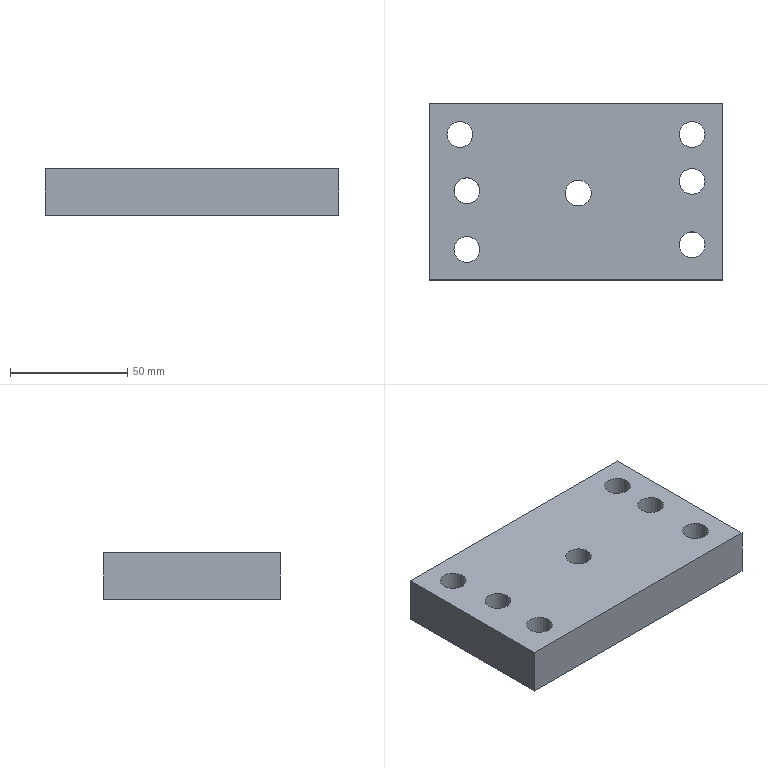Part | STEP file | 113_id2782_x_t | 1 solid | 13 faces | box 125 x 75 x 20 mm | volume 174195 mm3 | cylinder 7 | plane 6 | commonest cylinder face diameters 11 x7
STEP:
#1=CARTESIAN_POINT('',(0.,0.,0.));
#2=DIRECTION('',(0.,0.,1.));
#3=DIRECTION('',(1.,0.,0.));
#4=AXIS2_PLACEMENT_3D('',#1,#2,#3);
#5=CARTESIAN_POINT('',(1103.,139.,85.));
#6=VERTEX_POINT('',#5);
#7=CARTESIAN_POINT('',(1114.,139.,85.));
#8=VERTEX_POINT('',#7);
#9=CARTESIAN_POINT('',(1108.5,139.,85.));
#10=DIRECTION('',(0.,0.,1.));
#11=DIRECTION('',(-1.,0.,0.));
#12=AXIS2_PLACEMENT_3D('',#9,#10,#11);
#13=CIRCLE('',#12,5.5);
#14=CARTESIAN_POINT('',(1128.,155.,85.));
#15=DIRECTION('',(0.,0.,-1.));
#16=DIRECTION('',(1.,0.,0.));
#17=AXIS2_PLACEMENT_3D('',#14,#15,#16);
#18=PLANE('',#17);
#19=CARTESIAN_POINT('',(-25.,16.));
#20=CARTESIAN_POINT('',(-25.,25.526));
#21=CARTESIAN_POINT('',(-16.75,20.763));
#22=CARTESIAN_POINT('',(-8.5,16.));
#23=CARTESIAN_POINT('',(-16.75,11.237));
#24=CARTESIAN_POINT('',(-25.,6.474));
#25=CARTESIAN_POINT('',(-25.,16.));
#26=(BOUNDED_CURVE()B_SPLINE_CURVE(2,(#19,#20,#21,#22,#23,#24,#25),.UNSPECIFIED.,.T.,.F.)B_SPLINE_CURVE_WITH_KNOTS((1,2,2,2,2,1),(-2.094,0.,2.094,4.189,6.283,8.378),.UNSPECIFIED.)CURVE()GEOMETRIC_REPRESENTATION_ITEM()RATIONAL_B_SPLINE_CURVE((1.,0.5,1.,0.5,1.,0.5,1.))REPRESENTATION_ITEM(''));
#27=(GEOMETRIC_REPRESENTATION_CONTEXT(2)PARAMETRIC_REPRESENTATION_CONTEXT()REPRESENTATION_CONTEXT('',''));
#28=DEFINITIONAL_REPRESENTATION('',(#26),#27);
#29=PCURVE('',#18,#28);
#30=CARTESIAN_POINT('',(1108.5,139.,215.));
#31=DIRECTION('',(0.,0.,-1.));
#32=DIRECTION('',(1.,0.,0.));
#33=AXIS2_PLACEMENT_3D('',#30,#31,#32);
#34=CYLINDRICAL_SURFACE('',#33,5.5);
#35=CARTESIAN_POINT('',(3.142,130.));
#36=DIRECTION('',(-1.,0.));
#37=VECTOR('',#36,1.);
#38=LINE('',#35,#37);
#39=(GEOMETRIC_REPRESENTATION_CONTEXT(2)PARAMETRIC_REPRESENTATION_CONTEXT()REPRESENTATION_CONTEXT('',''));
#40=DEFINITIONAL_REPRESENTATION('',(#38),#39);
#41=PCURVE('',#34,#40);
#42=SURFACE_CURVE('',#13,(#29,#41),.PCURVE_S1.);
#43=EDGE_CURVE('',#6,#8,#42,.T.);
#44=ORIENTED_EDGE('',*,*,#43,.T.);
#45=CARTESIAN_POINT('',(1108.5,139.,85.));
#46=DIRECTION('',(0.,0.,1.));
#47=DIRECTION('',(-1.,0.,0.));
#48=AXIS2_PLACEMENT_3D('',#45,#46,#47);
#49=CIRCLE('',#48,5.5);
#50=CARTESIAN_POINT('',(-25.,16.));
#51=CARTESIAN_POINT('',(-25.,25.526));
#52=CARTESIAN_POINT('',(-16.75,20.763));
#53=CARTESIAN_POINT('',(-8.5,16.));
#54=CARTESIAN_POINT('',(-16.75,11.237));
#55=CARTESIAN_POINT('',(-25.,6.474));
#56=CARTESIAN_POINT('',(-25.,16.));
#57=(BOUNDED_CURVE()B_SPLINE_CURVE(2,(#50,#51,#52,#53,#54,#55,#56),.UNSPECIFIED.,.T.,.F.)B_SPLINE_CURVE_WITH_KNOTS((1,2,2,2,2,1),(-2.094,0.,2.094,4.189,6.283,8.378),.UNSPECIFIED.)CURVE()GEOMETRIC_REPRESENTATION_ITEM()RATIONAL_B_SPLINE_CURVE((1.,0.5,1.,0.5,1.,0.5,1.))REPRESENTATION_ITEM(''));
#58=(GEOMETRIC_REPRESENTATION_CONTEXT(2)PARAMETRIC_REPRESENTATION_CONTEXT()REPRESENTATION_CONTEXT('',''));
#59=DEFINITIONAL_REPRESENTATION('',(#57),#58);
#60=PCURVE('',#18,#59);
#61=CARTESIAN_POINT('',(9.425,130.));
#62=DIRECTION('',(-1.,0.));
#63=VECTOR('',#62,1.);
#64=LINE('',#61,#63);
#65=(GEOMETRIC_REPRESENTATION_CONTEXT(2)PARAMETRIC_REPRESENTATION_CONTEXT()REPRESENTATION_CONTEXT('',''));
#66=DEFINITIONAL_REPRESENTATION('',(#64),#65);
#67=PCURVE('',#34,#66);
#68=SURFACE_CURVE('',#49,(#60,#67),.PCURVE_S1.);
#69=EDGE_CURVE('',#8,#6,#68,.T.);
#70=ORIENTED_EDGE('',*,*,#69,.T.);
#71=EDGE_LOOP('',(#44,#70));
#72=FACE_BOUND('',#71,.T.);
#73=CARTESIAN_POINT('',(1054.5,161.,85.));
#74=VERTEX_POINT('',#73);
#75=CARTESIAN_POINT('',(1065.5,161.,85.));
#76=VERTEX_POINT('',#75);
#77=CARTESIAN_POINT('',(1060.,161.,85.));
#78=DIRECTION('',(0.,0.,1.));
#79=DIRECTION('',(-1.,0.,0.));
#80=AXIS2_PLACEMENT_3D('',#77,#78,#79);
#81=CIRCLE('',#80,5.5);
#82=CARTESIAN_POINT('',(-73.5,-6.));
#83=CARTESIAN_POINT('',(-73.5,3.526));
#84=CARTESIAN_POINT('',(-65.25,-1.237));
#85=CARTESIAN_POINT('',(-57.,-6.));
#86=CARTESIAN_POINT('',(-65.25,-10.763));
#87=CARTESIAN_POINT('',(-73.5,-15.526));
#88=CARTESIAN_POINT('',(-73.5,-6.));
#89=(BOUNDED_CURVE()B_SPLINE_CURVE(2,(#82,#83,#84,#85,#86,#87,#88),.UNSPECIFIED.,.T.,.F.)B_SPLINE_CURVE_WITH_KNOTS((1,2,2,2,2,1),(-2.094,0.,2.094,4.189,6.283,8.378),.UNSPECIFIED.)CURVE()GEOMETRIC_REPRESENTATION_ITEM()RATIONAL_B_SPLINE_CURVE((1.,0.5,1.,0.5,1.,0.5,1.))REPRESENTATION_ITEM(''));
#90=(GEOMETRIC_REPRESENTATION_CONTEXT(2)PARAMETRIC_REPRESENTATION_CONTEXT()REPRESENTATION_CONTEXT('',''));
#91=DEFINITIONAL_REPRESENTATION('',(#89),#90);
#92=PCURVE('',#18,#91);
#93=CARTESIAN_POINT('',(1060.,161.,190.));
#94=DIRECTION('',(0.,0.,-1.));
#95=DIRECTION('',(1.,0.,0.));
#96=AXIS2_PLACEMENT_3D('',#93,#94,#95);
#97=CYLINDRICAL_SURFACE('',#96,5.5);
#98=CARTESIAN_POINT('',(3.142,105.));
#99=DIRECTION('',(-1.,0.));
#100=VECTOR('',#99,1.);
#101=LINE('',#98,#100);
#102=(GEOMETRIC_REPRESENTATION_CONTEXT(2)PARAMETRIC_REPRESENTATION_CONTEXT()REPRESENTATION_CONTEXT('',''));
#103=DEFINITIONAL_REPRESENTATION('',(#101),#102);
#104=PCURVE('',#97,#103);
#105=SURFACE_CURVE('',#81,(#92,#104),.PCURVE_S1.);
#106=EDGE_CURVE('',#74,#76,#105,.T.);
#107=ORIENTED_EDGE('',*,*,#106,.T.);
#108=CARTESIAN_POINT('',(1060.,161.,85.));
#109=DIRECTION('',(0.,0.,1.));
#110=DIRECTION('',(-1.,0.,0.));
#111=AXIS2_PLACEMENT_3D('',#108,#109,#110);
#112=CIRCLE('',#111,5.5);
#113=CARTESIAN_POINT('',(-73.5,-6.));
#114=CARTESIAN_POINT('',(-73.5,3.526));
#115=CARTESIAN_POINT('',(-65.25,-1.237));
#116=CARTESIAN_POINT('',(-57.,-6.));
#117=CARTESIAN_POINT('',(-65.25,-10.763));
#118=CARTESIAN_POINT('',(-73.5,-15.526));
#119=CARTESIAN_POINT('',(-73.5,-6.));
#120=(BOUNDED_CURVE()B_SPLINE_CURVE(2,(#113,#114,#115,#116,#117,#118,#119),.UNSPECIFIED.,.T.,.F.)B_SPLINE_CURVE_WITH_KNOTS((1,2,2,2,2,1),(-2.094,0.,2.094,4.189,6.283,8.378),.UNSPECIFIED.)CURVE()GEOMETRIC_REPRESENTATION_ITEM()RATIONAL_B_SPLINE_CURVE((1.,0.5,1.,0.5,1.,0.5,1.))REPRESENTATION_ITEM(''));
#121=(GEOMETRIC_REPRESENTATION_CONTEXT(2)PARAMETRIC_REPRESENTATION_CONTEXT()REPRESENTATION_CONTEXT('',''));
#122=DEFINITIONAL_REPRESENTATION('',(#120),#121);
#123=PCURVE('',#18,#122);
#124=CARTESIAN_POINT('',(9.425,105.));
#125=DIRECTION('',(-1.,0.));
#126=VECTOR('',#125,1.);
#127=LINE('',#124,#126);
#128=(GEOMETRIC_REPRESENTATION_CONTEXT(2)PARAMETRIC_REPRESENTATION_CONTEXT()REPRESENTATION_CONTEXT('',''));
#129=DEFINITIONAL_REPRESENTATION('',(#127),#128);
#130=PCURVE('',#97,#129);
#131=SURFACE_CURVE('',#112,(#123,#130),.PCURVE_S1.);
#132=EDGE_CURVE('',#76,#74,#131,.T.);
#133=ORIENTED_EDGE('',*,*,#132,.T.);
#134=EDGE_LOOP('',(#107,#133));
#135=FACE_BOUND('',#134,.T.);
#136=CARTESIAN_POINT('',(1018.,137.,85.));
#137=VERTEX_POINT('',#136);
#138=CARTESIAN_POINT('',(1012.5,137.,85.));
#139=DIRECTION('',(0.,0.,1.));
#140=DIRECTION('',(-1.,0.,0.));
#141=AXIS2_PLACEMENT_3D('',#138,#139,#140);
#142=CIRCLE('',#141,5.5);
#143=CARTESIAN_POINT('',(-121.,18.));
#144=CARTESIAN_POINT('',(-121.,27.526));
#145=CARTESIAN_POINT('',(-112.75,22.763));
#146=CARTESIAN_POINT('',(-104.5,18.));
#147=CARTESIAN_POINT('',(-112.75,13.237));
#148=CARTESIAN_POINT('',(-121.,8.474));
#149=CARTESIAN_POINT('',(-121.,18.));
#150=(BOUNDED_CURVE()B_SPLINE_CURVE(2,(#143,#144,#145,#146,#147,#148,#149),.UNSPECIFIED.,.T.,.F.)B_SPLINE_CURVE_WITH_KNOTS((1,2,2,2,2,1),(-2.094,0.,2.094,4.189,6.283,8.378),.UNSPECIFIED.)CURVE()GEOMETRIC_REPRESENTATION_ITEM()RATIONAL_B_SPLINE_CURVE((1.,0.5,1.,0.5,1.,0.5,1.))REPRESENTATION_ITEM(''));
#151=(GEOMETRIC_REPRESENTATION_CONTEXT(2)PARAMETRIC_REPRESENTATION_CONTEXT()REPRESENTATION_CONTEXT('',''));
#152=DEFINITIONAL_REPRESENTATION('',(#150),#151);
#153=PCURVE('',#18,#152);
#154=CARTESIAN_POINT('',(1012.5,137.,90.));
#155=DIRECTION('',(0.,0.,1.));
#156=DIRECTION('',(-1.,0.,0.));
#157=AXIS2_PLACEMENT_3D('',#154,#155,#156);
#158=CYLINDRICAL_SURFACE('',#157,5.5);
#159=CARTESIAN_POINT('',(0.,-5.));
#160=DIRECTION('',(1.,0.));
#161=VECTOR('',#160,1.);
#162=LINE('',#159,#161);
#163=(GEOMETRIC_REPRESENTATION_CONTEXT(2)PARAMETRIC_REPRESENTATION_CONTEXT()REPRESENTATION_CONTEXT('',''));
#164=DEFINITIONAL_REPRESENTATION('',(#162),#163);
#165=PCURVE('',#158,#164);
#166=SURFACE_CURVE('',#142,(#153,#165),.PCURVE_S1.);
#167=EDGE_CURVE('',#137,#137,#166,.T.);
#168=ORIENTED_EDGE('',*,*,#167,.T.);
#169=EDGE_LOOP('',(#168));
#170=FACE_BOUND('',#169,.T.);
#171=CARTESIAN_POINT('',(1012.5,167.5,85.));
#172=VERTEX_POINT('',#171);
#173=CARTESIAN_POINT('',(1018.,162.,85.));
#174=VERTEX_POINT('',#173);
#175=CARTESIAN_POINT('',(1012.5,162.,85.));
#176=DIRECTION('',(0.,0.,1.));
#177=DIRECTION('',(-1.,0.,0.));
#178=AXIS2_PLACEMENT_3D('',#175,#176,#177);
#179=CIRCLE('',#178,5.5);
#180=CARTESIAN_POINT('',(-121.,-7.));
#181=CARTESIAN_POINT('',(-121.,2.526));
#182=CARTESIAN_POINT('',(-112.75,-2.237));
#183=CARTESIAN_POINT('',(-104.5,-7.));
#184=CARTESIAN_POINT('',(-112.75,-11.763));
#185=CARTESIAN_POINT('',(-121.,-16.526));
#186=CARTESIAN_POINT('',(-121.,-7.));
#187=(BOUNDED_CURVE()B_SPLINE_CURVE(2,(#180,#181,#182,#183,#184,#185,#186),.UNSPECIFIED.,.T.,.F.)B_SPLINE_CURVE_WITH_KNOTS((1,2,2,2,2,1),(-2.094,0.,2.094,4.189,6.283,8.378),.UNSPECIFIED.)CURVE()GEOMETRIC_REPRESENTATION_ITEM()RATIONAL_B_SPLINE_CURVE((1.,0.5,1.,0.5,1.,0.5,1.))REPRESENTATION_ITEM(''));
#188=(GEOMETRIC_REPRESENTATION_CONTEXT(2)PARAMETRIC_REPRESENTATION_CONTEXT()REPRESENTATION_CONTEXT('',''));
#189=DEFINITIONAL_REPRESENTATION('',(#187),#188);
#190=PCURVE('',#18,#189);
#191=CARTESIAN_POINT('',(1012.5,162.,90.));
#192=DIRECTION('',(0.,0.,1.));
#193=DIRECTION('',(0.,-1.,0.));
#194=AXIS2_PLACEMENT_3D('',#191,#192,#193);
#195=CYLINDRICAL_SURFACE('',#194,5.5);
#196=CARTESIAN_POINT('',(-1.571,-5.));
#197=DIRECTION('',(1.,0.));
#198=VECTOR('',#197,1.);
#199=LINE('',#196,#198);
#200=(GEOMETRIC_REPRESENTATION_CONTEXT(2)PARAMETRIC_REPRESENTATION_CONTEXT()REPRESENTATION_CONTEXT('',''));
#201=DEFINITIONAL_REPRESENTATION('',(#199),#200);
#202=PCURVE('',#195,#201);
#203=SURFACE_CURVE('',#179,(#190,#202),.PCURVE_S1.);
#204=EDGE_CURVE('',#172,#174,#203,.T.);
#205=ORIENTED_EDGE('',*,*,#204,.T.);
#206=CARTESIAN_POINT('',(1012.5,162.,85.));
#207=DIRECTION('',(0.,0.,1.));
#208=DIRECTION('',(-1.,0.,0.));
#209=AXIS2_PLACEMENT_3D('',#206,#207,#208);
#210=CIRCLE('',#209,5.5);
#211=CARTESIAN_POINT('',(-121.,-7.));
#212=CARTESIAN_POINT('',(-121.,2.526));
#213=CARTESIAN_POINT('',(-112.75,-2.237));
#214=CARTESIAN_POINT('',(-104.5,-7.));
#215=CARTESIAN_POINT('',(-112.75,-11.763));
#216=CARTESIAN_POINT('',(-121.,-16.526));
#217=CARTESIAN_POINT('',(-121.,-7.));
#218=(BOUNDED_CURVE()B_SPLINE_CURVE(2,(#211,#212,#213,#214,#215,#216,#217),.UNSPECIFIED.,.T.,.F.)B_SPLINE_CURVE_WITH_KNOTS((1,2,2,2,2,1),(-2.094,0.,2.094,4.189,6.283,8.378),.UNSPECIFIED.)CURVE()GEOMETRIC_REPRESENTATION_ITEM()RATIONAL_B_SPLINE_CURVE((1.,0.5,1.,0.5,1.,0.5,1.))REPRESENTATION_ITEM(''));
#219=(GEOMETRIC_REPRESENTATION_CONTEXT(2)PARAMETRIC_REPRESENTATION_CONTEXT()REPRESENTATION_CONTEXT('',''));
#220=DEFINITIONAL_REPRESENTATION('',(#218),#219);
#221=PCURVE('',#18,#220);
#222=CARTESIAN_POINT('',(-1.571,-5.));
#223=DIRECTION('',(1.,0.));
#224=VECTOR('',#223,1.);
#225=LINE('',#222,#224);
#226=(GEOMETRIC_REPRESENTATION_CONTEXT(2)PARAMETRIC_REPRESENTATION_CONTEXT()REPRESENTATION_CONTEXT('',''));
#227=DEFINITIONAL_REPRESENTATION('',(#225),#226);
#228=PCURVE('',#195,#227);
#229=SURFACE_CURVE('',#210,(#221,#228),.PCURVE_S1.);
#230=EDGE_CURVE('',#174,#172,#229,.T.);
#231=ORIENTED_EDGE('',*,*,#230,.T.);
#232=EDGE_LOOP('',(#205,#231));
#233=FACE_BOUND('',#232,.T.);
#234=CARTESIAN_POINT('',(1015.,186.,85.));
#235=VERTEX_POINT('',#234);
#236=CARTESIAN_POINT('',(1009.5,186.,85.));
#237=DIRECTION('',(0.,0.,1.));
#238=DIRECTION('',(-1.,0.,0.));
#239=AXIS2_PLACEMENT_3D('',#236,#237,#238);
#240=CIRCLE('',#239,5.5);
#241=CARTESIAN_POINT('',(-124.,-31.));
#242=CARTESIAN_POINT('',(-124.,-21.474));
#243=CARTESIAN_POINT('',(-115.75,-26.237));
#244=CARTESIAN_POINT('',(-107.5,-31.));
#245=CARTESIAN_POINT('',(-115.75,-35.763));
#246=CARTESIAN_POINT('',(-124.,-40.526));
#247=CARTESIAN_POINT('',(-124.,-31.));
#248=(BOUNDED_CURVE()B_SPLINE_CURVE(2,(#241,#242,#243,#244,#245,#246,#247),.UNSPECIFIED.,.T.,.F.)B_SPLINE_CURVE_WITH_KNOTS((1,2,2,2,2,1),(-2.094,0.,2.094,4.189,6.283,8.378),.UNSPECIFIED.)CURVE()GEOMETRIC_REPRESENTATION_ITEM()RATIONAL_B_SPLINE_CURVE((1.,0.5,1.,0.5,1.,0.5,1.))REPRESENTATION_ITEM(''));
#249=(GEOMETRIC_REPRESENTATION_CONTEXT(2)PARAMETRIC_REPRESENTATION_CONTEXT()REPRESENTATION_CONTEXT('',''));
#250=DEFINITIONAL_REPRESENTATION('',(#248),#249);
#251=PCURVE('',#18,#250);
#252=CARTESIAN_POINT('',(1009.5,186.,90.));
#253=DIRECTION('',(0.,0.,1.));
#254=DIRECTION('',(-1.,0.,0.));
#255=AXIS2_PLACEMENT_3D('',#252,#253,#254);
#256=CYLINDRICAL_SURFACE('',#255,5.5);
#257=CARTESIAN_POINT('',(0.,-5.));
#258=DIRECTION('',(1.,0.));
#259=VECTOR('',#258,1.);
#260=LINE('',#257,#259);
#261=(GEOMETRIC_REPRESENTATION_CONTEXT(2)PARAMETRIC_REPRESENTATION_CONTEXT()REPRESENTATION_CONTEXT('',''));
#262=DEFINITIONAL_REPRESENTATION('',(#260),#261);
#263=PCURVE('',#256,#262);
#264=SURFACE_CURVE('',#240,(#251,#263),.PCURVE_S1.);
#265=EDGE_CURVE('',#235,#235,#264,.T.);
#266=ORIENTED_EDGE('',*,*,#265,.T.);
#267=EDGE_LOOP('',(#266));
#268=FACE_BOUND('',#267,.T.);
#269=CARTESIAN_POINT('',(1121.5,199.,85.));
#270=VERTEX_POINT('',#269);
#271=CARTESIAN_POINT('',(1121.5,124.,85.));
#272=VERTEX_POINT('',#271);
#273=CARTESIAN_POINT('',(1121.5,155.,85.));
#274=DIRECTION('',(0.,-1.,0.));
#275=VECTOR('',#274,1.);
#276=LINE('',#273,#275);
#277=CARTESIAN_POINT('',(-6.5,0.));
#278=DIRECTION('',(0.,1.));
#279=VECTOR('',#278,1.);
#280=LINE('',#277,#279);
#281=(GEOMETRIC_REPRESENTATION_CONTEXT(2)PARAMETRIC_REPRESENTATION_CONTEXT()REPRESENTATION_CONTEXT('',''));
#282=DEFINITIONAL_REPRESENTATION('',(#280),#281);
#283=PCURVE('',#18,#282);
#284=CARTESIAN_POINT('',(1121.5,161.,38.5));
#285=DIRECTION('',(1.,0.,0.));
#286=DIRECTION('',(0.,0.,1.));
#287=AXIS2_PLACEMENT_3D('',#284,#285,#286);
#288=PLANE('',#287);
#289=CARTESIAN_POINT('',(46.5,6.));
#290=DIRECTION('',(0.,1.));
#291=VECTOR('',#290,1.);
#292=LINE('',#289,#291);
#293=(GEOMETRIC_REPRESENTATION_CONTEXT(2)PARAMETRIC_REPRESENTATION_CONTEXT()REPRESENTATION_CONTEXT('',''));
#294=DEFINITIONAL_REPRESENTATION('',(#292),#293);
#295=PCURVE('',#288,#294);
#296=SURFACE_CURVE('',#276,(#283,#295),.PCURVE_S1.);
#297=EDGE_CURVE('',#270,#272,#296,.T.);
#298=ORIENTED_EDGE('',*,*,#297,.T.);
#299=CARTESIAN_POINT('',(996.5,124.,85.));
#300=VERTEX_POINT('',#299);
#301=CARTESIAN_POINT('',(1128.,124.,85.));
#302=DIRECTION('',(1.,0.,0.));
#303=VECTOR('',#302,1.);
#304=LINE('',#301,#303);
#305=CARTESIAN_POINT('',(0.,31.));
#306=DIRECTION('',(1.,0.));
#307=VECTOR('',#306,1.);
#308=LINE('',#305,#307);
#309=(GEOMETRIC_REPRESENTATION_CONTEXT(2)PARAMETRIC_REPRESENTATION_CONTEXT()REPRESENTATION_CONTEXT('',''));
#310=DEFINITIONAL_REPRESENTATION('',(#308),#309);
#311=PCURVE('',#18,#310);
#312=CARTESIAN_POINT('',(1128.,124.,90.));
#313=DIRECTION('',(0.,-1.,0.));
#314=DIRECTION('',(0.,0.,1.));
#315=AXIS2_PLACEMENT_3D('',#312,#313,#314);
#316=PLANE('',#315);
#317=CARTESIAN_POINT('',(-5.,0.));
#318=DIRECTION('',(0.,-1.));
#319=VECTOR('',#318,1.);
#320=LINE('',#317,#319);
#321=(GEOMETRIC_REPRESENTATION_CONTEXT(2)PARAMETRIC_REPRESENTATION_CONTEXT()REPRESENTATION_CONTEXT('',''));
#322=DEFINITIONAL_REPRESENTATION('',(#320),#321);
#323=PCURVE('',#316,#322);
#324=SURFACE_CURVE('',#304,(#311,#323),.PCURVE_S1.);
#325=EDGE_CURVE('',#300,#272,#324,.T.);
#326=ORIENTED_EDGE('',*,*,#325,.F.);
#327=CARTESIAN_POINT('',(996.5,199.,85.));
#328=VERTEX_POINT('',#327);
#329=CARTESIAN_POINT('',(996.5,155.,85.));
#330=DIRECTION('',(0.,-1.,0.));
#331=VECTOR('',#330,1.);
#332=LINE('',#329,#331);
#333=CARTESIAN_POINT('',(-131.5,0.));
#334=DIRECTION('',(0.,1.));
#335=VECTOR('',#334,1.);
#336=LINE('',#333,#335);
#337=(GEOMETRIC_REPRESENTATION_CONTEXT(2)PARAMETRIC_REPRESENTATION_CONTEXT()REPRESENTATION_CONTEXT('',''));
#338=DEFINITIONAL_REPRESENTATION('',(#336),#337);
#339=PCURVE('',#18,#338);
#340=CARTESIAN_POINT('',(996.5,155.,90.));
#341=DIRECTION('',(-1.,0.,0.));
#342=DIRECTION('',(0.,0.,-1.));
#343=AXIS2_PLACEMENT_3D('',#340,#341,#342);
#344=PLANE('',#343);
#345=CARTESIAN_POINT('',(5.,0.));
#346=DIRECTION('',(0.,1.));
#347=VECTOR('',#346,1.);
#348=LINE('',#345,#347);
#349=(GEOMETRIC_REPRESENTATION_CONTEXT(2)PARAMETRIC_REPRESENTATION_CONTEXT()REPRESENTATION_CONTEXT('',''));
#350=DEFINITIONAL_REPRESENTATION('',(#348),#349);
#351=PCURVE('',#344,#350);
#352=SURFACE_CURVE('',#332,(#339,#351),.PCURVE_S1.);
#353=EDGE_CURVE('',#328,#300,#352,.T.);
#354=ORIENTED_EDGE('',*,*,#353,.F.);
#355=CARTESIAN_POINT('',(1128.,199.,85.));
#356=DIRECTION('',(-1.,0.,0.));
#357=VECTOR('',#356,1.);
#358=LINE('',#355,#357);
#359=CARTESIAN_POINT('',(0.,-44.));
#360=DIRECTION('',(-1.,0.));
#361=VECTOR('',#360,1.);
#362=LINE('',#359,#361);
#363=(GEOMETRIC_REPRESENTATION_CONTEXT(2)PARAMETRIC_REPRESENTATION_CONTEXT()REPRESENTATION_CONTEXT('',''));
#364=DEFINITIONAL_REPRESENTATION('',(#362),#363);
#365=PCURVE('',#18,#364);
#366=CARTESIAN_POINT('',(1128.,199.,90.));
#367=DIRECTION('',(0.,1.,0.));
#368=DIRECTION('',(0.,0.,-1.));
#369=AXIS2_PLACEMENT_3D('',#366,#367,#368);
#370=PLANE('',#369);
#371=CARTESIAN_POINT('',(5.,0.));
#372=DIRECTION('',(0.,1.));
#373=VECTOR('',#372,1.);
#374=LINE('',#371,#373);
#375=(GEOMETRIC_REPRESENTATION_CONTEXT(2)PARAMETRIC_REPRESENTATION_CONTEXT()REPRESENTATION_CONTEXT('',''));
#376=DEFINITIONAL_REPRESENTATION('',(#374),#375);
#377=PCURVE('',#370,#376);
#378=SURFACE_CURVE('',#358,(#365,#377),.PCURVE_S1.);
#379=EDGE_CURVE('',#270,#328,#378,.T.);
#380=ORIENTED_EDGE('',*,*,#379,.F.);
#381=EDGE_LOOP('',(#298,#326,#354,#380));
#382=FACE_BOUND('',#381,.T.);
#383=CARTESIAN_POINT('',(1103.,166.,85.));
#384=VERTEX_POINT('',#383);
#385=CARTESIAN_POINT('',(1114.,166.,85.));
#386=VERTEX_POINT('',#385);
#387=CARTESIAN_POINT('',(1108.5,166.,85.));
#388=DIRECTION('',(0.,0.,-1.));
#389=DIRECTION('',(-1.,0.,0.));
#390=AXIS2_PLACEMENT_3D('',#387,#388,#389);
#391=CIRCLE('',#390,5.5);
#392=CARTESIAN_POINT('',(-19.5,-11.));
#393=DIRECTION('',(-1.,0.));
#394=AXIS2_PLACEMENT_2D('',#392,#393);
#395=CIRCLE('',#394,5.5);
#396=(GEOMETRIC_REPRESENTATION_CONTEXT(2)PARAMETRIC_REPRESENTATION_CONTEXT()REPRESENTATION_CONTEXT('',''));
#397=DEFINITIONAL_REPRESENTATION('',(#395),#396);
#398=PCURVE('',#18,#397);
#399=CARTESIAN_POINT('',(1108.5,166.,200.));
#400=DIRECTION('',(0.,0.,-1.));
#401=DIRECTION('',(1.,0.,0.));
#402=AXIS2_PLACEMENT_3D('',#399,#400,#401);
#403=CYLINDRICAL_SURFACE('',#402,5.5);
#404=CARTESIAN_POINT('',(3.142,115.));
#405=DIRECTION('',(1.,0.));
#406=VECTOR('',#405,1.);
#407=LINE('',#404,#406);
#408=(GEOMETRIC_REPRESENTATION_CONTEXT(2)PARAMETRIC_REPRESENTATION_CONTEXT()REPRESENTATION_CONTEXT('',''));
#409=DEFINITIONAL_REPRESENTATION('',(#407),#408);
#410=PCURVE('',#403,#409);
#411=SURFACE_CURVE('',#391,(#398,#410),.PCURVE_S1.);
#412=EDGE_CURVE('',#384,#386,#411,.T.);
#413=ORIENTED_EDGE('',*,*,#412,.F.);
#414=CARTESIAN_POINT('',(1108.5,166.,85.));
#415=DIRECTION('',(0.,0.,-1.));
#416=DIRECTION('',(-1.,0.,0.));
#417=AXIS2_PLACEMENT_3D('',#414,#415,#416);
#418=CIRCLE('',#417,5.5);
#419=CARTESIAN_POINT('',(-19.5,-11.));
#420=DIRECTION('',(-1.,0.));
#421=AXIS2_PLACEMENT_2D('',#419,#420);
#422=CIRCLE('',#421,5.5);
#423=(GEOMETRIC_REPRESENTATION_CONTEXT(2)PARAMETRIC_REPRESENTATION_CONTEXT()REPRESENTATION_CONTEXT('',''));
#424=DEFINITIONAL_REPRESENTATION('',(#422),#423);
#425=PCURVE('',#18,#424);
#426=CARTESIAN_POINT('',(-3.142,115.));
#427=DIRECTION('',(1.,0.));
#428=VECTOR('',#427,1.);
#429=LINE('',#426,#428);
#430=(GEOMETRIC_REPRESENTATION_CONTEXT(2)PARAMETRIC_REPRESENTATION_CONTEXT()REPRESENTATION_CONTEXT('',''));
#431=DEFINITIONAL_REPRESENTATION('',(#429),#430);
#432=PCURVE('',#403,#431);
#433=SURFACE_CURVE('',#418,(#425,#432),.PCURVE_S1.);
#434=EDGE_CURVE('',#386,#384,#433,.T.);
#435=ORIENTED_EDGE('',*,*,#434,.F.);
#436=EDGE_LOOP('',(#413,#435));
#437=FACE_BOUND('',#436,.T.);
#438=CARTESIAN_POINT('',(1114.,186.,85.));
#439=VERTEX_POINT('',#438);
#440=CARTESIAN_POINT('',(1108.5,186.,85.));
#441=DIRECTION('',(0.,0.,1.));
#442=DIRECTION('',(-1.,0.,0.));
#443=AXIS2_PLACEMENT_3D('',#440,#441,#442);
#444=CIRCLE('',#443,5.5);
#445=CARTESIAN_POINT('',(-25.,-31.));
#446=CARTESIAN_POINT('',(-25.,-21.474));
#447=CARTESIAN_POINT('',(-16.75,-26.237));
#448=CARTESIAN_POINT('',(-8.5,-31.));
#449=CARTESIAN_POINT('',(-16.75,-35.763));
#450=CARTESIAN_POINT('',(-25.,-40.526));
#451=CARTESIAN_POINT('',(-25.,-31.));
#452=(BOUNDED_CURVE()B_SPLINE_CURVE(2,(#445,#446,#447,#448,#449,#450,#451),.UNSPECIFIED.,.T.,.F.)B_SPLINE_CURVE_WITH_KNOTS((1,2,2,2,2,1),(-2.094,0.,2.094,4.189,6.283,8.378),.UNSPECIFIED.)CURVE()GEOMETRIC_REPRESENTATION_ITEM()RATIONAL_B_SPLINE_CURVE((1.,0.5,1.,0.5,1.,0.5,1.))REPRESENTATION_ITEM(''));
#453=(GEOMETRIC_REPRESENTATION_CONTEXT(2)PARAMETRIC_REPRESENTATION_CONTEXT()REPRESENTATION_CONTEXT('',''));
#454=DEFINITIONAL_REPRESENTATION('',(#452),#453);
#455=PCURVE('',#18,#454);
#456=CARTESIAN_POINT('',(1108.5,186.,230.));
#457=DIRECTION('',(0.,0.,-1.));
#458=DIRECTION('',(1.,0.,0.));
#459=AXIS2_PLACEMENT_3D('',#456,#457,#458);
#460=CYLINDRICAL_SURFACE('',#459,5.5);
#461=CARTESIAN_POINT('',(9.425,145.));
#462=DIRECTION('',(-1.,0.));
#463=VECTOR('',#462,1.);
#464=LINE('',#461,#463);
#465=(GEOMETRIC_REPRESENTATION_CONTEXT(2)PARAMETRIC_REPRESENTATION_CONTEXT()REPRESENTATION_CONTEXT('',''));
#466=DEFINITIONAL_REPRESENTATION('',(#464),#465);
#467=PCURVE('',#460,#466);
#468=SURFACE_CURVE('',#444,(#455,#467),.PCURVE_S1.);
#469=EDGE_CURVE('',#439,#439,#468,.T.);
#470=ORIENTED_EDGE('',*,*,#469,.T.);
#471=EDGE_LOOP('',(#470));
#472=FACE_BOUND('',#471,.T.);
#473=ADVANCED_FACE('',(#72,#135,#170,#233,#268,#382,#437,#472),#18,.T.);
#474=CARTESIAN_POINT('',(1114.,139.,105.));
#475=VERTEX_POINT('',#474);
#476=CARTESIAN_POINT('',(1108.5,139.,105.));
#477=DIRECTION('',(0.,0.,-1.));
#478=DIRECTION('',(1.,0.,0.));
#479=AXIS2_PLACEMENT_3D('',#476,#477,#478);
#480=CIRCLE('',#479,5.5);
#481=CARTESIAN_POINT('',(1128.,155.,105.));
#482=DIRECTION('',(0.,0.,1.));
#483=DIRECTION('',(-1.,0.,0.));
#484=AXIS2_PLACEMENT_3D('',#481,#482,#483);
#485=PLANE('',#484);
#486=CARTESIAN_POINT('',(14.,16.));
#487=CARTESIAN_POINT('',(14.,25.526));
#488=CARTESIAN_POINT('',(22.25,20.763));
#489=CARTESIAN_POINT('',(30.5,16.));
#490=CARTESIAN_POINT('',(22.25,11.237));
#491=CARTESIAN_POINT('',(14.,6.474));
#492=CARTESIAN_POINT('',(14.,16.));
#493=(BOUNDED_CURVE()B_SPLINE_CURVE(2,(#486,#487,#488,#489,#490,#491,#492),.UNSPECIFIED.,.T.,.F.)B_SPLINE_CURVE_WITH_KNOTS((1,2,2,2,2,1),(-2.094,0.,2.094,4.189,6.283,8.378),.UNSPECIFIED.)CURVE()GEOMETRIC_REPRESENTATION_ITEM()RATIONAL_B_SPLINE_CURVE((1.,0.5,1.,0.5,1.,0.5,1.))REPRESENTATION_ITEM(''));
#494=(GEOMETRIC_REPRESENTATION_CONTEXT(2)PARAMETRIC_REPRESENTATION_CONTEXT()REPRESENTATION_CONTEXT('',''));
#495=DEFINITIONAL_REPRESENTATION('',(#493),#494);
#496=PCURVE('',#485,#495);
#497=CARTESIAN_POINT('',(0.,110.));
#498=DIRECTION('',(1.,0.));
#499=VECTOR('',#498,1.);
#500=LINE('',#497,#499);
#501=(GEOMETRIC_REPRESENTATION_CONTEXT(2)PARAMETRIC_REPRESENTATION_CONTEXT()REPRESENTATION_CONTEXT('',''));
#502=DEFINITIONAL_REPRESENTATION('',(#500),#501);
#503=PCURVE('',#34,#502);
#504=SURFACE_CURVE('',#480,(#496,#503),.PCURVE_S1.);
#505=EDGE_CURVE('',#475,#475,#504,.T.);
#506=ORIENTED_EDGE('',*,*,#505,.T.);
#507=EDGE_LOOP('',(#506));
#508=FACE_BOUND('',#507,.T.);
#509=CARTESIAN_POINT('',(1065.5,161.,105.));
#510=VERTEX_POINT('',#509);
#511=CARTESIAN_POINT('',(1060.,161.,105.));
#512=DIRECTION('',(0.,0.,-1.));
#513=DIRECTION('',(1.,0.,0.));
#514=AXIS2_PLACEMENT_3D('',#511,#512,#513);
#515=CIRCLE('',#514,5.5);
#516=CARTESIAN_POINT('',(62.5,-6.));
#517=CARTESIAN_POINT('',(62.5,3.526));
#518=CARTESIAN_POINT('',(70.75,-1.237));
#519=CARTESIAN_POINT('',(79.,-6.));
#520=CARTESIAN_POINT('',(70.75,-10.763));
#521=CARTESIAN_POINT('',(62.5,-15.526));
#522=CARTESIAN_POINT('',(62.5,-6.));
#523=(BOUNDED_CURVE()B_SPLINE_CURVE(2,(#516,#517,#518,#519,#520,#521,#522),.UNSPECIFIED.,.T.,.F.)B_SPLINE_CURVE_WITH_KNOTS((1,2,2,2,2,1),(-2.094,0.,2.094,4.189,6.283,8.378),.UNSPECIFIED.)CURVE()GEOMETRIC_REPRESENTATION_ITEM()RATIONAL_B_SPLINE_CURVE((1.,0.5,1.,0.5,1.,0.5,1.))REPRESENTATION_ITEM(''));
#524=(GEOMETRIC_REPRESENTATION_CONTEXT(2)PARAMETRIC_REPRESENTATION_CONTEXT()REPRESENTATION_CONTEXT('',''));
#525=DEFINITIONAL_REPRESENTATION('',(#523),#524);
#526=PCURVE('',#485,#525);
#527=CARTESIAN_POINT('',(0.,85.));
#528=DIRECTION('',(1.,0.));
#529=VECTOR('',#528,1.);
#530=LINE('',#527,#529);
#531=(GEOMETRIC_REPRESENTATION_CONTEXT(2)PARAMETRIC_REPRESENTATION_CONTEXT()REPRESENTATION_CONTEXT('',''));
#532=DEFINITIONAL_REPRESENTATION('',(#530),#531);
#533=PCURVE('',#97,#532);
#534=SURFACE_CURVE('',#515,(#526,#533),.PCURVE_S1.);
#535=EDGE_CURVE('',#510,#510,#534,.T.);
#536=ORIENTED_EDGE('',*,*,#535,.T.);
#537=EDGE_LOOP('',(#536));
#538=FACE_BOUND('',#537,.T.);
#539=CARTESIAN_POINT('',(1018.,137.,105.));
#540=VERTEX_POINT('',#539);
#541=CARTESIAN_POINT('',(1012.5,137.,105.));
#542=DIRECTION('',(0.,0.,-1.));
#543=DIRECTION('',(1.,0.,0.));
#544=AXIS2_PLACEMENT_3D('',#541,#542,#543);
#545=CIRCLE('',#544,5.5);
#546=CARTESIAN_POINT('',(110.,18.));
#547=CARTESIAN_POINT('',(110.,27.526));
#548=CARTESIAN_POINT('',(118.25,22.763));
#549=CARTESIAN_POINT('',(126.5,18.));
#550=CARTESIAN_POINT('',(118.25,13.237));
#551=CARTESIAN_POINT('',(110.,8.474));
#552=CARTESIAN_POINT('',(110.,18.));
#553=(BOUNDED_CURVE()B_SPLINE_CURVE(2,(#546,#547,#548,#549,#550,#551,#552),.UNSPECIFIED.,.T.,.F.)B_SPLINE_CURVE_WITH_KNOTS((1,2,2,2,2,1),(-2.094,0.,2.094,4.189,6.283,8.378),.UNSPECIFIED.)CURVE()GEOMETRIC_REPRESENTATION_ITEM()RATIONAL_B_SPLINE_CURVE((1.,0.5,1.,0.5,1.,0.5,1.))REPRESENTATION_ITEM(''));
#554=(GEOMETRIC_REPRESENTATION_CONTEXT(2)PARAMETRIC_REPRESENTATION_CONTEXT()REPRESENTATION_CONTEXT('',''));
#555=DEFINITIONAL_REPRESENTATION('',(#553),#554);
#556=PCURVE('',#485,#555);
#557=CARTESIAN_POINT('',(9.425,15.));
#558=DIRECTION('',(-1.,0.));
#559=VECTOR('',#558,1.);
#560=LINE('',#557,#559);
#561=(GEOMETRIC_REPRESENTATION_CONTEXT(2)PARAMETRIC_REPRESENTATION_CONTEXT()REPRESENTATION_CONTEXT('',''));
#562=DEFINITIONAL_REPRESENTATION('',(#560),#561);
#563=PCURVE('',#158,#562);
#564=SURFACE_CURVE('',#545,(#556,#563),.PCURVE_S1.);
#565=EDGE_CURVE('',#540,#540,#564,.T.);
#566=ORIENTED_EDGE('',*,*,#565,.T.);
#567=EDGE_LOOP('',(#566));
#568=FACE_BOUND('',#567,.T.);
#569=CARTESIAN_POINT('',(1015.,186.,105.));
#570=VERTEX_POINT('',#569);
#571=CARTESIAN_POINT('',(1009.5,186.,105.));
#572=DIRECTION('',(0.,0.,-1.));
#573=DIRECTION('',(1.,0.,0.));
#574=AXIS2_PLACEMENT_3D('',#571,#572,#573);
#575=CIRCLE('',#574,5.5);
#576=CARTESIAN_POINT('',(113.,-31.));
#577=CARTESIAN_POINT('',(113.,-21.474));
#578=CARTESIAN_POINT('',(121.25,-26.237));
#579=CARTESIAN_POINT('',(129.5,-31.));
#580=CARTESIAN_POINT('',(121.25,-35.763));
#581=CARTESIAN_POINT('',(113.,-40.526));
#582=CARTESIAN_POINT('',(113.,-31.));
#583=(BOUNDED_CURVE()B_SPLINE_CURVE(2,(#576,#577,#578,#579,#580,#581,#582),.UNSPECIFIED.,.T.,.F.)B_SPLINE_CURVE_WITH_KNOTS((1,2,2,2,2,1),(-2.094,0.,2.094,4.189,6.283,8.378),.UNSPECIFIED.)CURVE()GEOMETRIC_REPRESENTATION_ITEM()RATIONAL_B_SPLINE_CURVE((1.,0.5,1.,0.5,1.,0.5,1.))REPRESENTATION_ITEM(''));
#584=(GEOMETRIC_REPRESENTATION_CONTEXT(2)PARAMETRIC_REPRESENTATION_CONTEXT()REPRESENTATION_CONTEXT('',''));
#585=DEFINITIONAL_REPRESENTATION('',(#583),#584);
#586=PCURVE('',#485,#585);
#587=CARTESIAN_POINT('',(9.425,15.));
#588=DIRECTION('',(-1.,0.));
#589=VECTOR('',#588,1.);
#590=LINE('',#587,#589);
#591=(GEOMETRIC_REPRESENTATION_CONTEXT(2)PARAMETRIC_REPRESENTATION_CONTEXT()REPRESENTATION_CONTEXT('',''));
#592=DEFINITIONAL_REPRESENTATION('',(#590),#591);
#593=PCURVE('',#256,#592);
#594=SURFACE_CURVE('',#575,(#586,#593),.PCURVE_S1.);
#595=EDGE_CURVE('',#570,#570,#594,.T.);
#596=ORIENTED_EDGE('',*,*,#595,.T.);
#597=EDGE_LOOP('',(#596));
#598=FACE_BOUND('',#597,.T.);
#599=CARTESIAN_POINT('',(1018.,162.,105.));
#600=VERTEX_POINT('',#599);
#601=CARTESIAN_POINT('',(1012.5,162.,105.));
#602=DIRECTION('',(0.,0.,-1.));
#603=DIRECTION('',(1.,0.,0.));
#604=AXIS2_PLACEMENT_3D('',#601,#602,#603);
#605=CIRCLE('',#604,5.5);
#606=CARTESIAN_POINT('',(110.,-7.));
#607=CARTESIAN_POINT('',(110.,2.526));
#608=CARTESIAN_POINT('',(118.25,-2.237));
#609=CARTESIAN_POINT('',(126.5,-7.));
#610=CARTESIAN_POINT('',(118.25,-11.763));
#611=CARTESIAN_POINT('',(110.,-16.526));
#612=CARTESIAN_POINT('',(110.,-7.));
#613=(BOUNDED_CURVE()B_SPLINE_CURVE(2,(#606,#607,#608,#609,#610,#611,#612),.UNSPECIFIED.,.T.,.F.)B_SPLINE_CURVE_WITH_KNOTS((1,2,2,2,2,1),(-2.094,0.,2.094,4.189,6.283,8.378),.UNSPECIFIED.)CURVE()GEOMETRIC_REPRESENTATION_ITEM()RATIONAL_B_SPLINE_CURVE((1.,0.5,1.,0.5,1.,0.5,1.))REPRESENTATION_ITEM(''));
#614=(GEOMETRIC_REPRESENTATION_CONTEXT(2)PARAMETRIC_REPRESENTATION_CONTEXT()REPRESENTATION_CONTEXT('',''));
#615=DEFINITIONAL_REPRESENTATION('',(#613),#614);
#616=PCURVE('',#485,#615);
#617=CARTESIAN_POINT('',(7.854,15.));
#618=DIRECTION('',(-1.,0.));
#619=VECTOR('',#618,1.);
#620=LINE('',#617,#619);
#621=(GEOMETRIC_REPRESENTATION_CONTEXT(2)PARAMETRIC_REPRESENTATION_CONTEXT()REPRESENTATION_CONTEXT('',''));
#622=DEFINITIONAL_REPRESENTATION('',(#620),#621);
#623=PCURVE('',#195,#622);
#624=SURFACE_CURVE('',#605,(#616,#623),.PCURVE_S1.);
#625=EDGE_CURVE('',#600,#600,#624,.T.);
#626=ORIENTED_EDGE('',*,*,#625,.T.);
#627=EDGE_LOOP('',(#626));
#628=FACE_BOUND('',#627,.T.);
#629=CARTESIAN_POINT('',(1121.5,124.,105.));
#630=VERTEX_POINT('',#629);
#631=CARTESIAN_POINT('',(996.5,124.,105.));
#632=VERTEX_POINT('',#631);
#633=CARTESIAN_POINT('',(1128.,124.,105.));
#634=DIRECTION('',(-1.,0.,0.));
#635=VECTOR('',#634,1.);
#636=LINE('',#633,#635);
#637=CARTESIAN_POINT('',(0.,31.));
#638=DIRECTION('',(1.,0.));
#639=VECTOR('',#638,1.);
#640=LINE('',#637,#639);
#641=(GEOMETRIC_REPRESENTATION_CONTEXT(2)PARAMETRIC_REPRESENTATION_CONTEXT()REPRESENTATION_CONTEXT('',''));
#642=DEFINITIONAL_REPRESENTATION('',(#640),#641);
#643=PCURVE('',#485,#642);
#644=CARTESIAN_POINT('',(15.,0.));
#645=DIRECTION('',(0.,1.));
#646=VECTOR('',#645,1.);
#647=LINE('',#644,#646);
#648=(GEOMETRIC_REPRESENTATION_CONTEXT(2)PARAMETRIC_REPRESENTATION_CONTEXT()REPRESENTATION_CONTEXT('',''));
#649=DEFINITIONAL_REPRESENTATION('',(#647),#648);
#650=PCURVE('',#316,#649);
#651=SURFACE_CURVE('',#636,(#643,#650),.PCURVE_S1.);
#652=EDGE_CURVE('',#630,#632,#651,.T.);
#653=ORIENTED_EDGE('',*,*,#652,.F.);
#654=CARTESIAN_POINT('',(1121.5,199.,105.));
#655=VERTEX_POINT('',#654);
#656=CARTESIAN_POINT('',(1121.5,155.,105.));
#657=DIRECTION('',(0.,1.,0.));
#658=VECTOR('',#657,1.);
#659=LINE('',#656,#658);
#660=CARTESIAN_POINT('',(6.5,0.));
#661=DIRECTION('',(0.,-1.));
#662=VECTOR('',#661,1.);
#663=LINE('',#660,#662);
#664=(GEOMETRIC_REPRESENTATION_CONTEXT(2)PARAMETRIC_REPRESENTATION_CONTEXT()REPRESENTATION_CONTEXT('',''));
#665=DEFINITIONAL_REPRESENTATION('',(#663),#664);
#666=PCURVE('',#485,#665);
#667=CARTESIAN_POINT('',(66.5,6.));
#668=DIRECTION('',(0.,-1.));
#669=VECTOR('',#668,1.);
#670=LINE('',#667,#669);
#671=(GEOMETRIC_REPRESENTATION_CONTEXT(2)PARAMETRIC_REPRESENTATION_CONTEXT()REPRESENTATION_CONTEXT('',''));
#672=DEFINITIONAL_REPRESENTATION('',(#670),#671);
#673=PCURVE('',#288,#672);
#674=SURFACE_CURVE('',#659,(#666,#673),.PCURVE_S1.);
#675=EDGE_CURVE('',#630,#655,#674,.T.);
#676=ORIENTED_EDGE('',*,*,#675,.T.);
#677=CARTESIAN_POINT('',(996.5,199.,105.));
#678=VERTEX_POINT('',#677);
#679=CARTESIAN_POINT('',(1128.,199.,105.));
#680=DIRECTION('',(1.,0.,0.));
#681=VECTOR('',#680,1.);
#682=LINE('',#679,#681);
#683=CARTESIAN_POINT('',(0.,-44.));
#684=DIRECTION('',(-1.,0.));
#685=VECTOR('',#684,1.);
#686=LINE('',#683,#685);
#687=(GEOMETRIC_REPRESENTATION_CONTEXT(2)PARAMETRIC_REPRESENTATION_CONTEXT()REPRESENTATION_CONTEXT('',''));
#688=DEFINITIONAL_REPRESENTATION('',(#686),#687);
#689=PCURVE('',#485,#688);
#690=CARTESIAN_POINT('',(-15.,0.));
#691=DIRECTION('',(0.,-1.));
#692=VECTOR('',#691,1.);
#693=LINE('',#690,#692);
#694=(GEOMETRIC_REPRESENTATION_CONTEXT(2)PARAMETRIC_REPRESENTATION_CONTEXT()REPRESENTATION_CONTEXT('',''));
#695=DEFINITIONAL_REPRESENTATION('',(#693),#694);
#696=PCURVE('',#370,#695);
#697=SURFACE_CURVE('',#682,(#689,#696),.PCURVE_S1.);
#698=EDGE_CURVE('',#678,#655,#697,.T.);
#699=ORIENTED_EDGE('',*,*,#698,.F.);
#700=CARTESIAN_POINT('',(996.5,155.,105.));
#701=DIRECTION('',(0.,1.,0.));
#702=VECTOR('',#701,1.);
#703=LINE('',#700,#702);
#704=CARTESIAN_POINT('',(131.5,0.));
#705=DIRECTION('',(0.,-1.));
#706=VECTOR('',#705,1.);
#707=LINE('',#704,#706);
#708=(GEOMETRIC_REPRESENTATION_CONTEXT(2)PARAMETRIC_REPRESENTATION_CONTEXT()REPRESENTATION_CONTEXT('',''));
#709=DEFINITIONAL_REPRESENTATION('',(#707),#708);
#710=PCURVE('',#485,#709);
#711=CARTESIAN_POINT('',(-15.,0.));
#712=DIRECTION('',(0.,-1.));
#713=VECTOR('',#712,1.);
#714=LINE('',#711,#713);
#715=(GEOMETRIC_REPRESENTATION_CONTEXT(2)PARAMETRIC_REPRESENTATION_CONTEXT()REPRESENTATION_CONTEXT('',''));
#716=DEFINITIONAL_REPRESENTATION('',(#714),#715);
#717=PCURVE('',#344,#716);
#718=SURFACE_CURVE('',#703,(#710,#717),.PCURVE_S1.);
#719=EDGE_CURVE('',#632,#678,#718,.T.);
#720=ORIENTED_EDGE('',*,*,#719,.F.);
#721=EDGE_LOOP('',(#653,#676,#699,#720));
#722=FACE_BOUND('',#721,.T.);
#723=CARTESIAN_POINT('',(1114.,166.,105.));
#724=VERTEX_POINT('',#723);
#725=CARTESIAN_POINT('',(1108.5,166.,105.));
#726=DIRECTION('',(0.,0.,1.));
#727=DIRECTION('',(1.,0.,0.));
#728=AXIS2_PLACEMENT_3D('',#725,#726,#727);
#729=CIRCLE('',#728,5.5);
#730=CARTESIAN_POINT('',(19.5,-11.));
#731=DIRECTION('',(-1.,0.));
#732=AXIS2_PLACEMENT_2D('',#730,#731);
#733=CIRCLE('',#732,5.5);
#734=(GEOMETRIC_REPRESENTATION_CONTEXT(2)PARAMETRIC_REPRESENTATION_CONTEXT()REPRESENTATION_CONTEXT('',''));
#735=DEFINITIONAL_REPRESENTATION('',(#733),#734);
#736=PCURVE('',#485,#735);
#737=CARTESIAN_POINT('',(6.283,95.));
#738=DIRECTION('',(-1.,0.));
#739=VECTOR('',#738,1.);
#740=LINE('',#737,#739);
#741=(GEOMETRIC_REPRESENTATION_CONTEXT(2)PARAMETRIC_REPRESENTATION_CONTEXT()REPRESENTATION_CONTEXT('',''));
#742=DEFINITIONAL_REPRESENTATION('',(#740),#741);
#743=PCURVE('',#403,#742);
#744=SURFACE_CURVE('',#729,(#736,#743),.PCURVE_S1.);
#745=EDGE_CURVE('',#724,#724,#744,.T.);
#746=ORIENTED_EDGE('',*,*,#745,.F.);
#747=EDGE_LOOP('',(#746));
#748=FACE_BOUND('',#747,.T.);
#749=CARTESIAN_POINT('',(1114.,186.,105.));
#750=VERTEX_POINT('',#749);
#751=CARTESIAN_POINT('',(1108.5,186.,105.));
#752=DIRECTION('',(0.,0.,-1.));
#753=DIRECTION('',(1.,0.,0.));
#754=AXIS2_PLACEMENT_3D('',#751,#752,#753);
#755=CIRCLE('',#754,5.5);
#756=CARTESIAN_POINT('',(14.,-31.));
#757=CARTESIAN_POINT('',(14.,-21.474));
#758=CARTESIAN_POINT('',(22.25,-26.237));
#759=CARTESIAN_POINT('',(30.5,-31.));
#760=CARTESIAN_POINT('',(22.25,-35.763));
#761=CARTESIAN_POINT('',(14.,-40.526));
#762=CARTESIAN_POINT('',(14.,-31.));
#763=(BOUNDED_CURVE()B_SPLINE_CURVE(2,(#756,#757,#758,#759,#760,#761,#762),.UNSPECIFIED.,.T.,.F.)B_SPLINE_CURVE_WITH_KNOTS((1,2,2,2,2,1),(-2.094,0.,2.094,4.189,6.283,8.378),.UNSPECIFIED.)CURVE()GEOMETRIC_REPRESENTATION_ITEM()RATIONAL_B_SPLINE_CURVE((1.,0.5,1.,0.5,1.,0.5,1.))REPRESENTATION_ITEM(''));
#764=(GEOMETRIC_REPRESENTATION_CONTEXT(2)PARAMETRIC_REPRESENTATION_CONTEXT()REPRESENTATION_CONTEXT('',''));
#765=DEFINITIONAL_REPRESENTATION('',(#763),#764);
#766=PCURVE('',#485,#765);
#767=CARTESIAN_POINT('',(0.,125.));
#768=DIRECTION('',(1.,0.));
#769=VECTOR('',#768,1.);
#770=LINE('',#767,#769);
#771=(GEOMETRIC_REPRESENTATION_CONTEXT(2)PARAMETRIC_REPRESENTATION_CONTEXT()REPRESENTATION_CONTEXT('',''));
#772=DEFINITIONAL_REPRESENTATION('',(#770),#771);
#773=PCURVE('',#460,#772);
#774=SURFACE_CURVE('',#755,(#766,#773),.PCURVE_S1.);
#775=EDGE_CURVE('',#750,#750,#774,.T.);
#776=ORIENTED_EDGE('',*,*,#775,.T.);
#777=EDGE_LOOP('',(#776));
#778=FACE_BOUND('',#777,.T.);
#779=ADVANCED_FACE('',(#508,#538,#568,#598,#628,#722,#748,#778),#485,.T.);
#780=CARTESIAN_POINT('',(1121.5,124.,90.));
#781=DIRECTION('',(0.,0.,1.));
#782=VECTOR('',#781,1.);
#783=LINE('',#780,#782);
#784=CARTESIAN_POINT('',(51.5,37.));
#785=DIRECTION('',(1.,0.));
#786=VECTOR('',#785,1.);
#787=LINE('',#784,#786);
#788=(GEOMETRIC_REPRESENTATION_CONTEXT(2)PARAMETRIC_REPRESENTATION_CONTEXT()REPRESENTATION_CONTEXT('',''));
#789=DEFINITIONAL_REPRESENTATION('',(#787),#788);
#790=PCURVE('',#288,#789);
#791=CARTESIAN_POINT('',(0.,6.5));
#792=DIRECTION('',(1.,0.));
#793=VECTOR('',#792,1.);
#794=LINE('',#791,#793);
#795=(GEOMETRIC_REPRESENTATION_CONTEXT(2)PARAMETRIC_REPRESENTATION_CONTEXT()REPRESENTATION_CONTEXT('',''));
#796=DEFINITIONAL_REPRESENTATION('',(#794),#795);
#797=PCURVE('',#316,#796);
#798=SURFACE_CURVE('',#783,(#790,#797),.PCURVE_S1.);
#799=EDGE_CURVE('',#272,#630,#798,.T.);
#800=ORIENTED_EDGE('',*,*,#799,.F.);
#801=ORIENTED_EDGE('',*,*,#297,.F.);
#802=CARTESIAN_POINT('',(1121.5,199.,90.));
#803=DIRECTION('',(0.,0.,-1.));
#804=VECTOR('',#803,1.);
#805=LINE('',#802,#804);
#806=CARTESIAN_POINT('',(51.5,-38.));
#807=DIRECTION('',(-1.,0.));
#808=VECTOR('',#807,1.);
#809=LINE('',#806,#808);
#810=(GEOMETRIC_REPRESENTATION_CONTEXT(2)PARAMETRIC_REPRESENTATION_CONTEXT()REPRESENTATION_CONTEXT('',''));
#811=DEFINITIONAL_REPRESENTATION('',(#809),#810);
#812=PCURVE('',#288,#811);
#813=CARTESIAN_POINT('',(0.,6.5));
#814=DIRECTION('',(1.,0.));
#815=VECTOR('',#814,1.);
#816=LINE('',#813,#815);
#817=(GEOMETRIC_REPRESENTATION_CONTEXT(2)PARAMETRIC_REPRESENTATION_CONTEXT()REPRESENTATION_CONTEXT('',''));
#818=DEFINITIONAL_REPRESENTATION('',(#816),#817);
#819=PCURVE('',#370,#818);
#820=SURFACE_CURVE('',#805,(#812,#819),.PCURVE_S1.);
#821=EDGE_CURVE('',#655,#270,#820,.T.);
#822=ORIENTED_EDGE('',*,*,#821,.F.);
#823=ORIENTED_EDGE('',*,*,#675,.F.);
#824=EDGE_LOOP('',(#800,#801,#822,#823));
#825=FACE_BOUND('',#824,.T.);
#826=ADVANCED_FACE('',(#825),#288,.T.);
#827=ORIENTED_EDGE('',*,*,#625,.T.);
#828=CARTESIAN_POINT('',(1018.,162.,85.));
#829=CARTESIAN_POINT('',(1018.,162.,105.));
#830=B_SPLINE_CURVE_WITH_KNOTS('',1,(#828,#829),.UNSPECIFIED.,.F.,.F.,(2,2),(-5.,15.),.PIECEWISE_BEZIER_KNOTS.);
#831=CARTESIAN_POINT('',(1.571,0.));
#832=DIRECTION('',(0.,1.));
#833=VECTOR('',#832,1.);
#834=LINE('',#831,#833);
#835=(GEOMETRIC_REPRESENTATION_CONTEXT(2)PARAMETRIC_REPRESENTATION_CONTEXT()REPRESENTATION_CONTEXT('',''));
#836=DEFINITIONAL_REPRESENTATION('',(#834),#835);
#837=PCURVE('',#195,#836);
#838=CARTESIAN_POINT('',(7.854,0.));
#839=DIRECTION('',(0.,1.));
#840=VECTOR('',#839,1.);
#841=LINE('',#838,#840);
#842=(GEOMETRIC_REPRESENTATION_CONTEXT(2)PARAMETRIC_REPRESENTATION_CONTEXT()REPRESENTATION_CONTEXT('',''));
#843=DEFINITIONAL_REPRESENTATION('',(#841),#842);
#844=PCURVE('',#195,#843);
#845=SEAM_CURVE('',#830,(#837,#844),.PCURVE_S1.);
#846=EDGE_CURVE('',#174,#600,#845,.T.);
#847=ORIENTED_EDGE('',*,*,#846,.F.);
#848=ORIENTED_EDGE('',*,*,#230,.T.);
#849=ORIENTED_EDGE('',*,*,#204,.T.);
#850=ORIENTED_EDGE('',*,*,#846,.T.);
#851=EDGE_LOOP('',(#827,#847,#848,#849,#850));
#852=FACE_BOUND('',#851,.F.);
#853=ADVANCED_FACE('',(#852),#195,.F.);
#854=ORIENTED_EDGE('',*,*,#265,.T.);
#855=CARTESIAN_POINT('',(1015.,186.,85.));
#856=CARTESIAN_POINT('',(1015.,186.,105.));
#857=B_SPLINE_CURVE_WITH_KNOTS('',1,(#855,#856),.UNSPECIFIED.,.F.,.F.,(2,2),(-5.,15.),.PIECEWISE_BEZIER_KNOTS.);
#858=CARTESIAN_POINT('',(9.425,0.));
#859=DIRECTION('',(0.,1.));
#860=VECTOR('',#859,1.);
#861=LINE('',#858,#860);
#862=(GEOMETRIC_REPRESENTATION_CONTEXT(2)PARAMETRIC_REPRESENTATION_CONTEXT()REPRESENTATION_CONTEXT('',''));
#863=DEFINITIONAL_REPRESENTATION('',(#861),#862);
#864=PCURVE('',#256,#863);
#865=CARTESIAN_POINT('',(3.142,0.));
#866=DIRECTION('',(0.,1.));
#867=VECTOR('',#866,1.);
#868=LINE('',#865,#867);
#869=(GEOMETRIC_REPRESENTATION_CONTEXT(2)PARAMETRIC_REPRESENTATION_CONTEXT()REPRESENTATION_CONTEXT('',''));
#870=DEFINITIONAL_REPRESENTATION('',(#868),#869);
#871=PCURVE('',#256,#870);
#872=SEAM_CURVE('',#857,(#864,#871),.PCURVE_S1.);
#873=EDGE_CURVE('',#235,#570,#872,.T.);
#874=ORIENTED_EDGE('',*,*,#873,.T.);
#875=ORIENTED_EDGE('',*,*,#595,.T.);
#876=ORIENTED_EDGE('',*,*,#873,.F.);
#877=EDGE_LOOP('',(#854,#874,#875,#876));
#878=FACE_BOUND('',#877,.F.);
#879=ADVANCED_FACE('',(#878),#256,.F.);
#880=ORIENTED_EDGE('',*,*,#565,.T.);
#881=CARTESIAN_POINT('',(1018.,137.,85.));
#882=CARTESIAN_POINT('',(1018.,137.,105.));
#883=B_SPLINE_CURVE_WITH_KNOTS('',1,(#881,#882),.UNSPECIFIED.,.F.,.F.,(2,2),(-5.,15.),.PIECEWISE_BEZIER_KNOTS.);
#884=CARTESIAN_POINT('',(3.142,0.));
#885=DIRECTION('',(0.,1.));
#886=VECTOR('',#885,1.);
#887=LINE('',#884,#886);
#888=(GEOMETRIC_REPRESENTATION_CONTEXT(2)PARAMETRIC_REPRESENTATION_CONTEXT()REPRESENTATION_CONTEXT('',''));
#889=DEFINITIONAL_REPRESENTATION('',(#887),#888);
#890=PCURVE('',#158,#889);
#891=CARTESIAN_POINT('',(9.425,0.));
#892=DIRECTION('',(0.,1.));
#893=VECTOR('',#892,1.);
#894=LINE('',#891,#893);
#895=(GEOMETRIC_REPRESENTATION_CONTEXT(2)PARAMETRIC_REPRESENTATION_CONTEXT()REPRESENTATION_CONTEXT('',''));
#896=DEFINITIONAL_REPRESENTATION('',(#894),#895);
#897=PCURVE('',#158,#896);
#898=SEAM_CURVE('',#883,(#890,#897),.PCURVE_S1.);
#899=EDGE_CURVE('',#137,#540,#898,.T.);
#900=ORIENTED_EDGE('',*,*,#899,.F.);
#901=ORIENTED_EDGE('',*,*,#167,.T.);
#902=ORIENTED_EDGE('',*,*,#899,.T.);
#903=EDGE_LOOP('',(#880,#900,#901,#902));
#904=FACE_BOUND('',#903,.F.);
#905=ADVANCED_FACE('',(#904),#158,.F.);
#906=ORIENTED_EDGE('',*,*,#535,.T.);
#907=CARTESIAN_POINT('',(1065.5,161.,105.));
#908=CARTESIAN_POINT('',(1065.5,161.,85.));
#909=B_SPLINE_CURVE_WITH_KNOTS('',1,(#907,#908),.UNSPECIFIED.,.F.,.F.,(2,2),(85.,105.),.PIECEWISE_BEZIER_KNOTS.);
#910=CARTESIAN_POINT('',(6.283,0.));
#911=DIRECTION('',(0.,1.));
#912=VECTOR('',#911,1.);
#913=LINE('',#910,#912);
#914=(GEOMETRIC_REPRESENTATION_CONTEXT(2)PARAMETRIC_REPRESENTATION_CONTEXT()REPRESENTATION_CONTEXT('',''));
#915=DEFINITIONAL_REPRESENTATION('',(#913),#914);
#916=PCURVE('',#97,#915);
#917=CARTESIAN_POINT('',(0.,0.));
#918=DIRECTION('',(0.,1.));
#919=VECTOR('',#918,1.);
#920=LINE('',#917,#919);
#921=(GEOMETRIC_REPRESENTATION_CONTEXT(2)PARAMETRIC_REPRESENTATION_CONTEXT()REPRESENTATION_CONTEXT('',''));
#922=DEFINITIONAL_REPRESENTATION('',(#920),#921);
#923=PCURVE('',#97,#922);
#924=SEAM_CURVE('',#909,(#916,#923),.PCURVE_S1.);
#925=EDGE_CURVE('',#510,#76,#924,.T.);
#926=ORIENTED_EDGE('',*,*,#925,.T.);
#927=ORIENTED_EDGE('',*,*,#132,.T.);
#928=ORIENTED_EDGE('',*,*,#106,.T.);
#929=ORIENTED_EDGE('',*,*,#925,.F.);
#930=EDGE_LOOP('',(#906,#926,#927,#928,#929));
#931=FACE_BOUND('',#930,.F.);
#932=ADVANCED_FACE('',(#931),#97,.F.);
#933=CARTESIAN_POINT('',(996.5,124.,90.));
#934=DIRECTION('',(0.,0.,1.));
#935=VECTOR('',#934,1.);
#936=LINE('',#933,#935);
#937=CARTESIAN_POINT('',(0.,31.));
#938=DIRECTION('',(-1.,0.));
#939=VECTOR('',#938,1.);
#940=LINE('',#937,#939);
#941=(GEOMETRIC_REPRESENTATION_CONTEXT(2)PARAMETRIC_REPRESENTATION_CONTEXT()REPRESENTATION_CONTEXT('',''));
#942=DEFINITIONAL_REPRESENTATION('',(#940),#941);
#943=PCURVE('',#344,#942);
#944=CARTESIAN_POINT('',(0.,131.5));
#945=DIRECTION('',(1.,0.));
#946=VECTOR('',#945,1.);
#947=LINE('',#944,#946);
#948=(GEOMETRIC_REPRESENTATION_CONTEXT(2)PARAMETRIC_REPRESENTATION_CONTEXT()REPRESENTATION_CONTEXT('',''));
#949=DEFINITIONAL_REPRESENTATION('',(#947),#948);
#950=PCURVE('',#316,#949);
#951=SURFACE_CURVE('',#936,(#943,#950),.PCURVE_S1.);
#952=EDGE_CURVE('',#300,#632,#951,.T.);
#953=ORIENTED_EDGE('',*,*,#952,.T.);
#954=ORIENTED_EDGE('',*,*,#719,.T.);
#955=CARTESIAN_POINT('',(996.5,199.,90.));
#956=DIRECTION('',(0.,0.,1.));
#957=VECTOR('',#956,1.);
#958=LINE('',#955,#957);
#959=CARTESIAN_POINT('',(0.,-44.));
#960=DIRECTION('',(-1.,0.));
#961=VECTOR('',#960,1.);
#962=LINE('',#959,#961);
#963=(GEOMETRIC_REPRESENTATION_CONTEXT(2)PARAMETRIC_REPRESENTATION_CONTEXT()REPRESENTATION_CONTEXT('',''));
#964=DEFINITIONAL_REPRESENTATION('',(#962),#963);
#965=PCURVE('',#344,#964);
#966=CARTESIAN_POINT('',(0.,131.5));
#967=DIRECTION('',(-1.,0.));
#968=VECTOR('',#967,1.);
#969=LINE('',#966,#968);
#970=(GEOMETRIC_REPRESENTATION_CONTEXT(2)PARAMETRIC_REPRESENTATION_CONTEXT()REPRESENTATION_CONTEXT('',''));
#971=DEFINITIONAL_REPRESENTATION('',(#969),#970);
#972=PCURVE('',#370,#971);
#973=SURFACE_CURVE('',#958,(#965,#972),.PCURVE_S1.);
#974=EDGE_CURVE('',#328,#678,#973,.T.);
#975=ORIENTED_EDGE('',*,*,#974,.F.);
#976=ORIENTED_EDGE('',*,*,#353,.T.);
#977=EDGE_LOOP('',(#953,#954,#975,#976));
#978=FACE_BOUND('',#977,.T.);
#979=ADVANCED_FACE('',(#978),#344,.T.);
#980=ORIENTED_EDGE('',*,*,#698,.T.);
#981=ORIENTED_EDGE('',*,*,#821,.T.);
#982=ORIENTED_EDGE('',*,*,#379,.T.);
#983=ORIENTED_EDGE('',*,*,#974,.T.);
#984=EDGE_LOOP('',(#980,#981,#982,#983));
#985=FACE_BOUND('',#984,.T.);
#986=ADVANCED_FACE('',(#985),#370,.T.);
#987=ORIENTED_EDGE('',*,*,#325,.T.);
#988=ORIENTED_EDGE('',*,*,#799,.T.);
#989=ORIENTED_EDGE('',*,*,#652,.T.);
#990=ORIENTED_EDGE('',*,*,#952,.F.);
#991=EDGE_LOOP('',(#987,#988,#989,#990));
#992=FACE_BOUND('',#991,.T.);
#993=ADVANCED_FACE('',(#992),#316,.T.);
#994=ORIENTED_EDGE('',*,*,#505,.T.);
#995=CARTESIAN_POINT('',(1114.,139.,105.));
#996=CARTESIAN_POINT('',(1114.,139.,85.));
#997=B_SPLINE_CURVE_WITH_KNOTS('',1,(#995,#996),.UNSPECIFIED.,.F.,.F.,(2,2),(110.,130.),.PIECEWISE_BEZIER_KNOTS.);
#998=CARTESIAN_POINT('',(6.283,0.));
#999=DIRECTION('',(0.,1.));
#1000=VECTOR('',#999,1.);
#1001=LINE('',#998,#1000);
#1002=(GEOMETRIC_REPRESENTATION_CONTEXT(2)PARAMETRIC_REPRESENTATION_CONTEXT()REPRESENTATION_CONTEXT('',''));
#1003=DEFINITIONAL_REPRESENTATION('',(#1001),#1002);
#1004=PCURVE('',#34,#1003);
#1005=CARTESIAN_POINT('',(0.,0.));
#1006=DIRECTION('',(0.,1.));
#1007=VECTOR('',#1006,1.);
#1008=LINE('',#1005,#1007);
#1009=(GEOMETRIC_REPRESENTATION_CONTEXT(2)PARAMETRIC_REPRESENTATION_CONTEXT()REPRESENTATION_CONTEXT('',''));
#1010=DEFINITIONAL_REPRESENTATION('',(#1008),#1009);
#1011=PCURVE('',#34,#1010);
#1012=SEAM_CURVE('',#997,(#1004,#1011),.PCURVE_S1.);
#1013=EDGE_CURVE('',#475,#8,#1012,.T.);
#1014=ORIENTED_EDGE('',*,*,#1013,.T.);
#1015=ORIENTED_EDGE('',*,*,#69,.T.);
#1016=ORIENTED_EDGE('',*,*,#43,.T.);
#1017=ORIENTED_EDGE('',*,*,#1013,.F.);
#1018=EDGE_LOOP('',(#994,#1014,#1015,#1016,#1017));
#1019=FACE_BOUND('',#1018,.F.);
#1020=ADVANCED_FACE('',(#1019),#34,.F.);
#1021=ORIENTED_EDGE('',*,*,#745,.F.);
#1022=CARTESIAN_POINT('',(1114.,166.,105.));
#1023=CARTESIAN_POINT('',(1114.,166.,85.));
#1024=B_SPLINE_CURVE_WITH_KNOTS('',1,(#1022,#1023),.UNSPECIFIED.,.F.,.F.,(2,2),(95.,115.),.PIECEWISE_BEZIER_KNOTS.);
#1025=CARTESIAN_POINT('',(6.283,0.));
#1026=DIRECTION('',(0.,1.));
#1027=VECTOR('',#1026,1.);
#1028=LINE('',#1025,#1027);
#1029=(GEOMETRIC_REPRESENTATION_CONTEXT(2)PARAMETRIC_REPRESENTATION_CONTEXT()REPRESENTATION_CONTEXT('',''));
#1030=DEFINITIONAL_REPRESENTATION('',(#1028),#1029);
#1031=PCURVE('',#403,#1030);
#1032=CARTESIAN_POINT('',(0.,0.));
#1033=DIRECTION('',(0.,1.));
#1034=VECTOR('',#1033,1.);
#1035=LINE('',#1032,#1034);
#1036=(GEOMETRIC_REPRESENTATION_CONTEXT(2)PARAMETRIC_REPRESENTATION_CONTEXT()REPRESENTATION_CONTEXT('',''));
#1037=DEFINITIONAL_REPRESENTATION('',(#1035),#1036);
#1038=PCURVE('',#403,#1037);
#1039=SEAM_CURVE('',#1024,(#1031,#1038),.PCURVE_S1.);
#1040=EDGE_CURVE('',#724,#386,#1039,.T.);
#1041=ORIENTED_EDGE('',*,*,#1040,.T.);
#1042=ORIENTED_EDGE('',*,*,#412,.F.);
#1043=ORIENTED_EDGE('',*,*,#434,.F.);
#1044=ORIENTED_EDGE('',*,*,#1040,.F.);
#1045=EDGE_LOOP('',(#1021,#1041,#1042,#1043,#1044));
#1046=FACE_BOUND('',#1045,.F.);
#1047=ADVANCED_FACE('',(#1046),#403,.F.);
#1048=ORIENTED_EDGE('',*,*,#775,.T.);
#1049=CARTESIAN_POINT('',(1114.,186.,105.));
#1050=CARTESIAN_POINT('',(1114.,186.,85.));
#1051=B_SPLINE_CURVE_WITH_KNOTS('',1,(#1049,#1050),.UNSPECIFIED.,.F.,.F.,(2,2),(125.,145.),.PIECEWISE_BEZIER_KNOTS.);
#1052=CARTESIAN_POINT('',(6.283,0.));
#1053=DIRECTION('',(0.,1.));
#1054=VECTOR('',#1053,1.);
#1055=LINE('',#1052,#1054);
#1056=(GEOMETRIC_REPRESENTATION_CONTEXT(2)PARAMETRIC_REPRESENTATION_CONTEXT()REPRESENTATION_CONTEXT('',''));
#1057=DEFINITIONAL_REPRESENTATION('',(#1055),#1056);
#1058=PCURVE('',#460,#1057);
#1059=CARTESIAN_POINT('',(0.,0.));
#1060=DIRECTION('',(0.,1.));
#1061=VECTOR('',#1060,1.);
#1062=LINE('',#1059,#1061);
#1063=(GEOMETRIC_REPRESENTATION_CONTEXT(2)PARAMETRIC_REPRESENTATION_CONTEXT()REPRESENTATION_CONTEXT('',''));
#1064=DEFINITIONAL_REPRESENTATION('',(#1062),#1063);
#1065=PCURVE('',#460,#1064);
#1066=SEAM_CURVE('',#1051,(#1058,#1065),.PCURVE_S1.);
#1067=EDGE_CURVE('',#750,#439,#1066,.T.);
#1068=ORIENTED_EDGE('',*,*,#1067,.T.);
#1069=ORIENTED_EDGE('',*,*,#469,.T.);
#1070=ORIENTED_EDGE('',*,*,#1067,.F.);
#1071=EDGE_LOOP('',(#1048,#1068,#1069,#1070));
#1072=FACE_BOUND('',#1071,.F.);
#1073=ADVANCED_FACE('',(#1072),#460,.F.);
#1074=CLOSED_SHELL('',(#473,#779,#826,#853,#879,#905,#932,#979,#986,#993,#1020,#1047,#1073));
#1075=MANIFOLD_SOLID_BREP('',#1074);
#1076=(LENGTH_UNIT()NAMED_UNIT(*)SI_UNIT(.MILLI.,.METRE.));
#1077=UNCERTAINTY_MEASURE_WITH_UNIT(LENGTH_MEASURE(0.000005),#1076,'','');
#1078=(NAMED_UNIT(*)PLANE_ANGLE_UNIT()SI_UNIT($,.RADIAN.));
#1079=(NAMED_UNIT(*)SI_UNIT($,.STERADIAN.)SOLID_ANGLE_UNIT());
#1080=(GEOMETRIC_REPRESENTATION_CONTEXT(3)GLOBAL_UNCERTAINTY_ASSIGNED_CONTEXT((#1077))GLOBAL_UNIT_ASSIGNED_CONTEXT((#1076,#1078,#1079))REPRESENTATION_CONTEXT('',''));
#1081=ADVANCED_BREP_SHAPE_REPRESENTATION('',(#4,#1075),#1080);